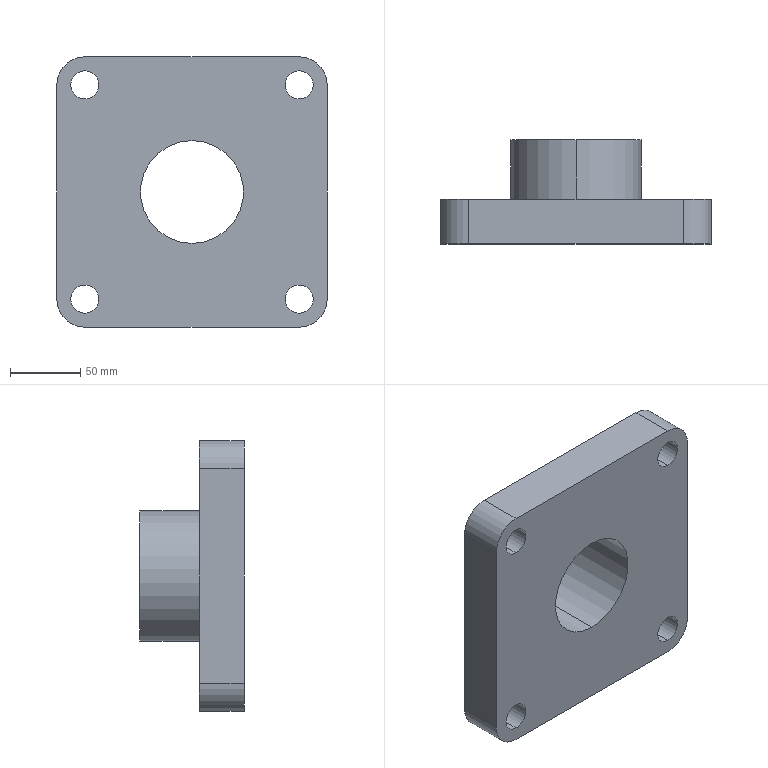Part | SolidWorks | features BaseBody 1 | 1 solid | 23 faces | box 193 x 74.6 x 193 mm | volume 1117041 mm3 | cylinder 16 | plane 7 | commonest cylinder face diameters 20 x8 40 x4 73.374 x2 93.374 x2
STEP:
#1=CARTESIAN_POINT('',(0.,74.6,-36.687));
#2=VERTEX_POINT('',#1);
#3=CARTESIAN_POINT('',(0.,74.6,36.687));
#4=VERTEX_POINT('',#3);
#5=CARTESIAN_POINT('',(0.,74.6,0.));
#6=DIRECTION('',(0.,1.,0.));
#7=DIRECTION('',(0.,0.,1.));
#8=AXIS2_PLACEMENT_3D('',#5,#6,#7);
#9=CIRCLE('',#8,36.687);
#10=EDGE_CURVE('',#2,#4,#9,.T.);
#11=ORIENTED_EDGE('',*,*,#10,.T.);
#12=CARTESIAN_POINT('',(0.,0.,36.687));
#13=VERTEX_POINT('',#12);
#14=CARTESIAN_POINT('',(0.,74.6,36.687));
#15=DIRECTION('',(0.,-1.,0.));
#16=VECTOR('',#15,1000.);
#17=LINE('',#14,#16);
#18=EDGE_CURVE('',#4,#13,#17,.T.);
#19=ORIENTED_EDGE('',*,*,#18,.T.);
#20=CARTESIAN_POINT('',(0.,0.,-36.687));
#21=VERTEX_POINT('',#20);
#22=CARTESIAN_POINT('',(0.,0.,0.));
#23=DIRECTION('',(0.,1.,0.));
#24=DIRECTION('',(0.,0.,1.));
#25=AXIS2_PLACEMENT_3D('',#22,#23,#24);
#26=CIRCLE('',#25,36.687);
#27=EDGE_CURVE('',#21,#13,#26,.T.);
#28=ORIENTED_EDGE('',*,*,#27,.F.);
#29=CARTESIAN_POINT('',(0.,74.6,-36.687));
#30=DIRECTION('',(0.,-1.,0.));
#31=VECTOR('',#30,1000.);
#32=LINE('',#29,#31);
#33=EDGE_CURVE('',#2,#21,#32,.T.);
#34=ORIENTED_EDGE('',*,*,#33,.F.);
#35=EDGE_LOOP('',(#11,#19,#28,#34));
#36=FACE_OUTER_BOUND('',#35,.T.);
#37=CARTESIAN_POINT('',(0.,74.6,0.));
#38=DIRECTION('',(0.,-1.,0.));
#39=DIRECTION('',(0.,0.,-1.));
#40=AXIS2_PLACEMENT_3D('',#37,#38,#39);
#41=CYLINDRICAL_SURFACE('',#40,36.687);
#42=ADVANCED_FACE('',(#36),#41,.F.);
#43=CARTESIAN_POINT('',(0.,74.6,46.687));
#44=VERTEX_POINT('',#43);
#45=CARTESIAN_POINT('',(0.,74.6,-46.687));
#46=VERTEX_POINT('',#45);
#47=CARTESIAN_POINT('',(0.,74.6,0.));
#48=DIRECTION('',(0.,1.,0.));
#49=DIRECTION('',(0.,0.,1.));
#50=AXIS2_PLACEMENT_3D('',#47,#48,#49);
#51=CIRCLE('',#50,46.687);
#52=EDGE_CURVE('',#44,#46,#51,.T.);
#53=ORIENTED_EDGE('',*,*,#52,.F.);
#54=CARTESIAN_POINT('',(0.,32.,46.687));
#55=VERTEX_POINT('',#54);
#56=CARTESIAN_POINT('',(0.,74.6,46.687));
#57=DIRECTION('',(0.,-1.,0.));
#58=VECTOR('',#57,1000.);
#59=LINE('',#56,#58);
#60=EDGE_CURVE('',#44,#55,#59,.T.);
#61=ORIENTED_EDGE('',*,*,#60,.T.);
#62=CARTESIAN_POINT('',(0.,32.,-46.687));
#63=VERTEX_POINT('',#62);
#64=CARTESIAN_POINT('',(0.,32.,0.));
#65=DIRECTION('',(0.,-1.,0.));
#66=DIRECTION('',(0.,0.,1.));
#67=AXIS2_PLACEMENT_3D('',#64,#65,#66);
#68=CIRCLE('',#67,46.687);
#69=EDGE_CURVE('',#63,#55,#68,.T.);
#70=ORIENTED_EDGE('',*,*,#69,.F.);
#71=CARTESIAN_POINT('',(0.,74.6,-46.687));
#72=DIRECTION('',(0.,-1.,0.));
#73=VECTOR('',#72,1000.);
#74=LINE('',#71,#73);
#75=EDGE_CURVE('',#46,#63,#74,.T.);
#76=ORIENTED_EDGE('',*,*,#75,.F.);
#77=EDGE_LOOP('',(#53,#61,#70,#76));
#78=FACE_OUTER_BOUND('',#77,.T.);
#79=CARTESIAN_POINT('',(0.,74.6,0.));
#80=DIRECTION('',(0.,-1.,0.));
#81=DIRECTION('',(0.,0.,-1.));
#82=AXIS2_PLACEMENT_3D('',#79,#80,#81);
#83=CYLINDRICAL_SURFACE('',#82,46.687);
#84=ADVANCED_FACE('',(#78),#83,.T.);
#85=CARTESIAN_POINT('',(76.5,32.,66.5));
#86=VERTEX_POINT('',#85);
#87=CARTESIAN_POINT('',(76.5,32.,86.5));
#88=VERTEX_POINT('',#87);
#89=CARTESIAN_POINT('',(76.5,32.,76.5));
#90=DIRECTION('',(0.,1.,0.));
#91=DIRECTION('',(0.,0.,1.));
#92=AXIS2_PLACEMENT_3D('',#89,#90,#91);
#93=CIRCLE('',#92,10.);
#94=EDGE_CURVE('',#86,#88,#93,.T.);
#95=ORIENTED_EDGE('',*,*,#94,.T.);
#96=CARTESIAN_POINT('',(76.5,0.,86.5));
#97=VERTEX_POINT('',#96);
#98=CARTESIAN_POINT('',(76.5,32.,86.5));
#99=DIRECTION('',(0.,-1.,0.));
#100=VECTOR('',#99,1000.);
#101=LINE('',#98,#100);
#102=EDGE_CURVE('',#88,#97,#101,.T.);
#103=ORIENTED_EDGE('',*,*,#102,.T.);
#104=CARTESIAN_POINT('',(76.5,0.,66.5));
#105=VERTEX_POINT('',#104);
#106=CARTESIAN_POINT('',(76.5,0.,76.5));
#107=DIRECTION('',(0.,1.,0.));
#108=DIRECTION('',(0.,0.,1.));
#109=AXIS2_PLACEMENT_3D('',#106,#107,#108);
#110=CIRCLE('',#109,10.);
#111=EDGE_CURVE('',#105,#97,#110,.T.);
#112=ORIENTED_EDGE('',*,*,#111,.F.);
#113=CARTESIAN_POINT('',(76.5,32.,66.5));
#114=DIRECTION('',(0.,-1.,0.));
#115=VECTOR('',#114,1000.);
#116=LINE('',#113,#115);
#117=EDGE_CURVE('',#86,#105,#116,.T.);
#118=ORIENTED_EDGE('',*,*,#117,.F.);
#119=EDGE_LOOP('',(#95,#103,#112,#118));
#120=FACE_OUTER_BOUND('',#119,.T.);
#121=CARTESIAN_POINT('',(76.5,32.,76.5));
#122=DIRECTION('',(0.,-1.,0.));
#123=DIRECTION('',(0.,0.,-1.));
#124=AXIS2_PLACEMENT_3D('',#121,#122,#123);
#125=CYLINDRICAL_SURFACE('',#124,10.);
#126=ADVANCED_FACE('',(#120),#125,.F.);
#127=CARTESIAN_POINT('',(76.5,32.,-86.5));
#128=VERTEX_POINT('',#127);
#129=CARTESIAN_POINT('',(76.5,32.,-66.5));
#130=VERTEX_POINT('',#129);
#131=CARTESIAN_POINT('',(76.5,32.,-76.5));
#132=DIRECTION('',(0.,1.,0.));
#133=DIRECTION('',(0.,0.,1.));
#134=AXIS2_PLACEMENT_3D('',#131,#132,#133);
#135=CIRCLE('',#134,10.);
#136=EDGE_CURVE('',#128,#130,#135,.T.);
#137=ORIENTED_EDGE('',*,*,#136,.T.);
#138=CARTESIAN_POINT('',(76.5,0.,-66.5));
#139=VERTEX_POINT('',#138);
#140=CARTESIAN_POINT('',(76.5,32.,-66.5));
#141=DIRECTION('',(0.,-1.,0.));
#142=VECTOR('',#141,1000.);
#143=LINE('',#140,#142);
#144=EDGE_CURVE('',#130,#139,#143,.T.);
#145=ORIENTED_EDGE('',*,*,#144,.T.);
#146=CARTESIAN_POINT('',(76.5,0.,-86.5));
#147=VERTEX_POINT('',#146);
#148=CARTESIAN_POINT('',(76.5,0.,-76.5));
#149=DIRECTION('',(0.,1.,0.));
#150=DIRECTION('',(0.,0.,1.));
#151=AXIS2_PLACEMENT_3D('',#148,#149,#150);
#152=CIRCLE('',#151,10.);
#153=EDGE_CURVE('',#147,#139,#152,.T.);
#154=ORIENTED_EDGE('',*,*,#153,.F.);
#155=CARTESIAN_POINT('',(76.5,32.,-86.5));
#156=DIRECTION('',(0.,-1.,0.));
#157=VECTOR('',#156,1000.);
#158=LINE('',#155,#157);
#159=EDGE_CURVE('',#128,#147,#158,.T.);
#160=ORIENTED_EDGE('',*,*,#159,.F.);
#161=EDGE_LOOP('',(#137,#145,#154,#160));
#162=FACE_OUTER_BOUND('',#161,.T.);
#163=CARTESIAN_POINT('',(76.5,32.,-76.5));
#164=DIRECTION('',(0.,-1.,0.));
#165=DIRECTION('',(0.,0.,-1.));
#166=AXIS2_PLACEMENT_3D('',#163,#164,#165);
#167=CYLINDRICAL_SURFACE('',#166,10.);
#168=ADVANCED_FACE('',(#162),#167,.F.);
#169=CARTESIAN_POINT('',(-76.5,32.,66.5));
#170=VERTEX_POINT('',#169);
#171=CARTESIAN_POINT('',(-76.5,32.,86.5));
#172=VERTEX_POINT('',#171);
#173=CARTESIAN_POINT('',(-76.5,32.,76.5));
#174=DIRECTION('',(0.,1.,0.));
#175=DIRECTION('',(0.,0.,1.));
#176=AXIS2_PLACEMENT_3D('',#173,#174,#175);
#177=CIRCLE('',#176,10.);
#178=EDGE_CURVE('',#170,#172,#177,.T.);
#179=ORIENTED_EDGE('',*,*,#178,.T.);
#180=CARTESIAN_POINT('',(-76.5,0.,86.5));
#181=VERTEX_POINT('',#180);
#182=CARTESIAN_POINT('',(-76.5,32.,86.5));
#183=DIRECTION('',(0.,-1.,0.));
#184=VECTOR('',#183,1000.);
#185=LINE('',#182,#184);
#186=EDGE_CURVE('',#172,#181,#185,.T.);
#187=ORIENTED_EDGE('',*,*,#186,.T.);
#188=CARTESIAN_POINT('',(-76.5,0.,66.5));
#189=VERTEX_POINT('',#188);
#190=CARTESIAN_POINT('',(-76.5,0.,76.5));
#191=DIRECTION('',(0.,1.,0.));
#192=DIRECTION('',(0.,0.,1.));
#193=AXIS2_PLACEMENT_3D('',#190,#191,#192);
#194=CIRCLE('',#193,10.);
#195=EDGE_CURVE('',#189,#181,#194,.T.);
#196=ORIENTED_EDGE('',*,*,#195,.F.);
#197=CARTESIAN_POINT('',(-76.5,32.,66.5));
#198=DIRECTION('',(0.,-1.,0.));
#199=VECTOR('',#198,1000.);
#200=LINE('',#197,#199);
#201=EDGE_CURVE('',#170,#189,#200,.T.);
#202=ORIENTED_EDGE('',*,*,#201,.F.);
#203=EDGE_LOOP('',(#179,#187,#196,#202));
#204=FACE_OUTER_BOUND('',#203,.T.);
#205=CARTESIAN_POINT('',(-76.5,32.,76.5));
#206=DIRECTION('',(0.,-1.,0.));
#207=DIRECTION('',(0.,0.,-1.));
#208=AXIS2_PLACEMENT_3D('',#205,#206,#207);
#209=CYLINDRICAL_SURFACE('',#208,10.);
#210=ADVANCED_FACE('',(#204),#209,.F.);
#211=CARTESIAN_POINT('',(-76.5,32.,-86.5));
#212=VERTEX_POINT('',#211);
#213=CARTESIAN_POINT('',(-76.5,32.,-66.5));
#214=VERTEX_POINT('',#213);
#215=CARTESIAN_POINT('',(-76.5,32.,-76.5));
#216=DIRECTION('',(0.,1.,0.));
#217=DIRECTION('',(0.,0.,1.));
#218=AXIS2_PLACEMENT_3D('',#215,#216,#217);
#219=CIRCLE('',#218,10.);
#220=EDGE_CURVE('',#212,#214,#219,.T.);
#221=ORIENTED_EDGE('',*,*,#220,.T.);
#222=CARTESIAN_POINT('',(-76.5,0.,-66.5));
#223=VERTEX_POINT('',#222);
#224=CARTESIAN_POINT('',(-76.5,32.,-66.5));
#225=DIRECTION('',(0.,-1.,0.));
#226=VECTOR('',#225,1000.);
#227=LINE('',#224,#226);
#228=EDGE_CURVE('',#214,#223,#227,.T.);
#229=ORIENTED_EDGE('',*,*,#228,.T.);
#230=CARTESIAN_POINT('',(-76.5,0.,-86.5));
#231=VERTEX_POINT('',#230);
#232=CARTESIAN_POINT('',(-76.5,0.,-76.5));
#233=DIRECTION('',(0.,1.,0.));
#234=DIRECTION('',(0.,0.,1.));
#235=AXIS2_PLACEMENT_3D('',#232,#233,#234);
#236=CIRCLE('',#235,10.);
#237=EDGE_CURVE('',#231,#223,#236,.T.);
#238=ORIENTED_EDGE('',*,*,#237,.F.);
#239=CARTESIAN_POINT('',(-76.5,32.,-86.5));
#240=DIRECTION('',(0.,-1.,0.));
#241=VECTOR('',#240,1000.);
#242=LINE('',#239,#241);
#243=EDGE_CURVE('',#212,#231,#242,.T.);
#244=ORIENTED_EDGE('',*,*,#243,.F.);
#245=EDGE_LOOP('',(#221,#229,#238,#244));
#246=FACE_OUTER_BOUND('',#245,.T.);
#247=CARTESIAN_POINT('',(-76.5,32.,-76.5));
#248=DIRECTION('',(0.,-1.,0.));
#249=DIRECTION('',(0.,0.,-1.));
#250=AXIS2_PLACEMENT_3D('',#247,#248,#249);
#251=CYLINDRICAL_SURFACE('',#250,10.);
#252=ADVANCED_FACE('',(#246),#251,.F.);
#253=ORIENTED_EDGE('',*,*,#69,.T.);
#254=CARTESIAN_POINT('',(0.,32.,0.));
#255=DIRECTION('',(0.,-1.,0.));
#256=DIRECTION('',(0.,0.,1.));
#257=AXIS2_PLACEMENT_3D('',#254,#255,#256);
#258=CIRCLE('',#257,46.687);
#259=EDGE_CURVE('',#55,#63,#258,.T.);
#260=ORIENTED_EDGE('',*,*,#259,.T.);
#261=EDGE_LOOP('',(#253,#260));
#262=FACE_BOUND('',#261,.T.);
#263=ORIENTED_EDGE('',*,*,#136,.F.);
#264=CARTESIAN_POINT('',(76.5,32.,-76.5));
#265=DIRECTION('',(0.,1.,0.));
#266=DIRECTION('',(0.,0.,1.));
#267=AXIS2_PLACEMENT_3D('',#264,#265,#266);
#268=CIRCLE('',#267,10.);
#269=EDGE_CURVE('',#130,#128,#268,.T.);
#270=ORIENTED_EDGE('',*,*,#269,.F.);
#271=EDGE_LOOP('',(#263,#270));
#272=FACE_BOUND('',#271,.T.);
#273=ORIENTED_EDGE('',*,*,#220,.F.);
#274=CARTESIAN_POINT('',(-76.5,32.,-76.5));
#275=DIRECTION('',(0.,1.,0.));
#276=DIRECTION('',(0.,0.,1.));
#277=AXIS2_PLACEMENT_3D('',#274,#275,#276);
#278=CIRCLE('',#277,10.);
#279=EDGE_CURVE('',#214,#212,#278,.T.);
#280=ORIENTED_EDGE('',*,*,#279,.F.);
#281=EDGE_LOOP('',(#273,#280));
#282=FACE_BOUND('',#281,.T.);
#283=CARTESIAN_POINT('',(-76.5,32.,-96.5));
#284=VERTEX_POINT('',#283);
#285=CARTESIAN_POINT('',(-96.5,32.,-76.5));
#286=VERTEX_POINT('',#285);
#287=CARTESIAN_POINT('',(-76.5,32.,-76.5));
#288=DIRECTION('',(0.,1.,0.));
#289=DIRECTION('',(0.,0.,1.));
#290=AXIS2_PLACEMENT_3D('',#287,#288,#289);
#291=CIRCLE('',#290,20.);
#292=EDGE_CURVE('',#284,#286,#291,.T.);
#293=ORIENTED_EDGE('',*,*,#292,.T.);
#294=CARTESIAN_POINT('',(-96.5,32.,76.5));
#295=VERTEX_POINT('',#294);
#296=CARTESIAN_POINT('',(-96.5,32.,-76.5));
#297=DIRECTION('',(0.,0.,1.));
#298=VECTOR('',#297,1000.);
#299=LINE('',#296,#298);
#300=EDGE_CURVE('',#286,#295,#299,.T.);
#301=ORIENTED_EDGE('',*,*,#300,.T.);
#302=CARTESIAN_POINT('',(-76.5,32.,96.5));
#303=VERTEX_POINT('',#302);
#304=CARTESIAN_POINT('',(-76.5,32.,76.5));
#305=DIRECTION('',(0.,1.,0.));
#306=DIRECTION('',(0.,0.,-1.));
#307=AXIS2_PLACEMENT_3D('',#304,#305,#306);
#308=CIRCLE('',#307,20.);
#309=EDGE_CURVE('',#295,#303,#308,.T.);
#310=ORIENTED_EDGE('',*,*,#309,.T.);
#311=CARTESIAN_POINT('',(76.5,32.,96.5));
#312=VERTEX_POINT('',#311);
#313=CARTESIAN_POINT('',(-76.5,32.,96.5));
#314=DIRECTION('',(1.,0.,0.));
#315=VECTOR('',#314,1000.);
#316=LINE('',#313,#315);
#317=EDGE_CURVE('',#303,#312,#316,.T.);
#318=ORIENTED_EDGE('',*,*,#317,.T.);
#319=CARTESIAN_POINT('',(96.5,32.,76.5));
#320=VERTEX_POINT('',#319);
#321=CARTESIAN_POINT('',(76.5,32.,76.5));
#322=DIRECTION('',(0.,1.,0.));
#323=DIRECTION('',(0.,0.,1.));
#324=AXIS2_PLACEMENT_3D('',#321,#322,#323);
#325=CIRCLE('',#324,20.);
#326=EDGE_CURVE('',#312,#320,#325,.T.);
#327=ORIENTED_EDGE('',*,*,#326,.T.);
#328=CARTESIAN_POINT('',(96.5,32.,-76.5));
#329=VERTEX_POINT('',#328);
#330=CARTESIAN_POINT('',(96.5,32.,-76.5));
#331=DIRECTION('',(0.,0.,-1.));
#332=VECTOR('',#331,1000.);
#333=LINE('',#330,#332);
#334=EDGE_CURVE('',#320,#329,#333,.T.);
#335=ORIENTED_EDGE('',*,*,#334,.T.);
#336=CARTESIAN_POINT('',(76.5,32.,-96.5));
#337=VERTEX_POINT('',#336);
#338=CARTESIAN_POINT('',(76.5,32.,-76.5));
#339=DIRECTION('',(0.,1.,0.));
#340=DIRECTION('',(0.,0.,1.));
#341=AXIS2_PLACEMENT_3D('',#338,#339,#340);
#342=CIRCLE('',#341,20.);
#343=EDGE_CURVE('',#329,#337,#342,.T.);
#344=ORIENTED_EDGE('',*,*,#343,.T.);
#345=CARTESIAN_POINT('',(-76.5,32.,-96.5));
#346=DIRECTION('',(-1.,0.,0.));
#347=VECTOR('',#346,1000.);
#348=LINE('',#345,#347);
#349=EDGE_CURVE('',#337,#284,#348,.T.);
#350=ORIENTED_EDGE('',*,*,#349,.T.);
#351=EDGE_LOOP('',(#293,#301,#310,#318,#327,#335,#344,#350));
#352=FACE_OUTER_BOUND('',#351,.T.);
#353=ORIENTED_EDGE('',*,*,#178,.F.);
#354=CARTESIAN_POINT('',(-76.5,32.,76.5));
#355=DIRECTION('',(0.,1.,0.));
#356=DIRECTION('',(0.,0.,1.));
#357=AXIS2_PLACEMENT_3D('',#354,#355,#356);
#358=CIRCLE('',#357,10.);
#359=EDGE_CURVE('',#172,#170,#358,.T.);
#360=ORIENTED_EDGE('',*,*,#359,.F.);
#361=EDGE_LOOP('',(#353,#360));
#362=FACE_BOUND('',#361,.T.);
#363=ORIENTED_EDGE('',*,*,#94,.F.);
#364=CARTESIAN_POINT('',(76.5,32.,76.5));
#365=DIRECTION('',(0.,1.,0.));
#366=DIRECTION('',(0.,0.,1.));
#367=AXIS2_PLACEMENT_3D('',#364,#365,#366);
#368=CIRCLE('',#367,10.);
#369=EDGE_CURVE('',#88,#86,#368,.T.);
#370=ORIENTED_EDGE('',*,*,#369,.F.);
#371=EDGE_LOOP('',(#363,#370));
#372=FACE_BOUND('',#371,.T.);
#373=CARTESIAN_POINT('',(-76.5,32.,-76.5));
#374=DIRECTION('',(0.,1.,0.));
#375=DIRECTION('',(0.,0.,1.));
#376=AXIS2_PLACEMENT_3D('',#373,#374,#375);
#377=PLANE('',#376);
#378=ADVANCED_FACE('',(#262,#272,#282,#352,#362,#372),#377,.T.);
#379=ORIENTED_EDGE('',*,*,#27,.T.);
#380=CARTESIAN_POINT('',(0.,0.,0.));
#381=DIRECTION('',(0.,1.,0.));
#382=DIRECTION('',(0.,0.,1.));
#383=AXIS2_PLACEMENT_3D('',#380,#381,#382);
#384=CIRCLE('',#383,36.687);
#385=EDGE_CURVE('',#13,#21,#384,.T.);
#386=ORIENTED_EDGE('',*,*,#385,.T.);
#387=EDGE_LOOP('',(#379,#386));
#388=FACE_BOUND('',#387,.T.);
#389=CARTESIAN_POINT('',(-76.5,0.,-96.5));
#390=VERTEX_POINT('',#389);
#391=CARTESIAN_POINT('',(-96.5,0.,-76.5));
#392=VERTEX_POINT('',#391);
#393=CARTESIAN_POINT('',(-76.5,0.,-76.5));
#394=DIRECTION('',(0.,1.,0.));
#395=DIRECTION('',(0.,0.,1.));
#396=AXIS2_PLACEMENT_3D('',#393,#394,#395);
#397=CIRCLE('',#396,20.);
#398=EDGE_CURVE('',#390,#392,#397,.T.);
#399=ORIENTED_EDGE('',*,*,#398,.F.);
#400=CARTESIAN_POINT('',(76.5,0.,-96.5));
#401=VERTEX_POINT('',#400);
#402=CARTESIAN_POINT('',(-76.5,0.,-96.5));
#403=DIRECTION('',(-1.,0.,0.));
#404=VECTOR('',#403,1000.);
#405=LINE('',#402,#404);
#406=EDGE_CURVE('',#401,#390,#405,.T.);
#407=ORIENTED_EDGE('',*,*,#406,.F.);
#408=CARTESIAN_POINT('',(96.5,0.,-76.5));
#409=VERTEX_POINT('',#408);
#410=CARTESIAN_POINT('',(76.5,0.,-76.5));
#411=DIRECTION('',(0.,1.,0.));
#412=DIRECTION('',(0.,0.,1.));
#413=AXIS2_PLACEMENT_3D('',#410,#411,#412);
#414=CIRCLE('',#413,20.);
#415=EDGE_CURVE('',#409,#401,#414,.T.);
#416=ORIENTED_EDGE('',*,*,#415,.F.);
#417=CARTESIAN_POINT('',(96.5,0.,76.5));
#418=VERTEX_POINT('',#417);
#419=CARTESIAN_POINT('',(96.5,0.,-76.5));
#420=DIRECTION('',(0.,0.,-1.));
#421=VECTOR('',#420,1000.);
#422=LINE('',#419,#421);
#423=EDGE_CURVE('',#418,#409,#422,.T.);
#424=ORIENTED_EDGE('',*,*,#423,.F.);
#425=CARTESIAN_POINT('',(76.5,0.,96.5));
#426=VERTEX_POINT('',#425);
#427=CARTESIAN_POINT('',(76.5,0.,76.5));
#428=DIRECTION('',(0.,1.,0.));
#429=DIRECTION('',(0.,0.,1.));
#430=AXIS2_PLACEMENT_3D('',#427,#428,#429);
#431=CIRCLE('',#430,20.);
#432=EDGE_CURVE('',#426,#418,#431,.T.);
#433=ORIENTED_EDGE('',*,*,#432,.F.);
#434=CARTESIAN_POINT('',(-76.5,0.,96.5));
#435=VERTEX_POINT('',#434);
#436=CARTESIAN_POINT('',(-76.5,0.,96.5));
#437=DIRECTION('',(1.,0.,0.));
#438=VECTOR('',#437,1000.);
#439=LINE('',#436,#438);
#440=EDGE_CURVE('',#435,#426,#439,.T.);
#441=ORIENTED_EDGE('',*,*,#440,.F.);
#442=CARTESIAN_POINT('',(-96.5,0.,76.5));
#443=VERTEX_POINT('',#442);
#444=CARTESIAN_POINT('',(-76.5,0.,76.5));
#445=DIRECTION('',(0.,1.,0.));
#446=DIRECTION('',(0.,0.,-1.));
#447=AXIS2_PLACEMENT_3D('',#444,#445,#446);
#448=CIRCLE('',#447,20.);
#449=EDGE_CURVE('',#443,#435,#448,.T.);
#450=ORIENTED_EDGE('',*,*,#449,.F.);
#451=CARTESIAN_POINT('',(-96.5,0.,-76.5));
#452=DIRECTION('',(0.,0.,1.));
#453=VECTOR('',#452,1000.);
#454=LINE('',#451,#453);
#455=EDGE_CURVE('',#392,#443,#454,.T.);
#456=ORIENTED_EDGE('',*,*,#455,.F.);
#457=EDGE_LOOP('',(#399,#407,#416,#424,#433,#441,#450,#456));
#458=FACE_OUTER_BOUND('',#457,.T.);
#459=ORIENTED_EDGE('',*,*,#237,.T.);
#460=CARTESIAN_POINT('',(-76.5,0.,-76.5));
#461=DIRECTION('',(0.,1.,0.));
#462=DIRECTION('',(0.,0.,1.));
#463=AXIS2_PLACEMENT_3D('',#460,#461,#462);
#464=CIRCLE('',#463,10.);
#465=EDGE_CURVE('',#223,#231,#464,.T.);
#466=ORIENTED_EDGE('',*,*,#465,.T.);
#467=EDGE_LOOP('',(#459,#466));
#468=FACE_BOUND('',#467,.T.);
#469=ORIENTED_EDGE('',*,*,#195,.T.);
#470=CARTESIAN_POINT('',(-76.5,0.,76.5));
#471=DIRECTION('',(0.,1.,0.));
#472=DIRECTION('',(0.,0.,1.));
#473=AXIS2_PLACEMENT_3D('',#470,#471,#472);
#474=CIRCLE('',#473,10.);
#475=EDGE_CURVE('',#181,#189,#474,.T.);
#476=ORIENTED_EDGE('',*,*,#475,.T.);
#477=EDGE_LOOP('',(#469,#476));
#478=FACE_BOUND('',#477,.T.);
#479=ORIENTED_EDGE('',*,*,#153,.T.);
#480=CARTESIAN_POINT('',(76.5,0.,-76.5));
#481=DIRECTION('',(0.,1.,0.));
#482=DIRECTION('',(0.,0.,1.));
#483=AXIS2_PLACEMENT_3D('',#480,#481,#482);
#484=CIRCLE('',#483,10.);
#485=EDGE_CURVE('',#139,#147,#484,.T.);
#486=ORIENTED_EDGE('',*,*,#485,.T.);
#487=EDGE_LOOP('',(#479,#486));
#488=FACE_BOUND('',#487,.T.);
#489=ORIENTED_EDGE('',*,*,#111,.T.);
#490=CARTESIAN_POINT('',(76.5,0.,76.5));
#491=DIRECTION('',(0.,1.,0.));
#492=DIRECTION('',(0.,0.,1.));
#493=AXIS2_PLACEMENT_3D('',#490,#491,#492);
#494=CIRCLE('',#493,10.);
#495=EDGE_CURVE('',#97,#105,#494,.T.);
#496=ORIENTED_EDGE('',*,*,#495,.T.);
#497=EDGE_LOOP('',(#489,#496));
#498=FACE_BOUND('',#497,.T.);
#499=CARTESIAN_POINT('',(-76.5,0.,-76.5));
#500=DIRECTION('',(0.,1.,0.));
#501=DIRECTION('',(0.,0.,1.));
#502=AXIS2_PLACEMENT_3D('',#499,#500,#501);
#503=PLANE('',#502);
#504=ADVANCED_FACE('',(#388,#458,#468,#478,#488,#498),#503,.F.);
#505=ORIENTED_EDGE('',*,*,#398,.T.);
#506=CARTESIAN_POINT('',(-96.5,32.,-76.5));
#507=DIRECTION('',(0.,-1.,0.));
#508=VECTOR('',#507,1000.);
#509=LINE('',#506,#508);
#510=EDGE_CURVE('',#286,#392,#509,.T.);
#511=ORIENTED_EDGE('',*,*,#510,.F.);
#512=ORIENTED_EDGE('',*,*,#292,.F.);
#513=CARTESIAN_POINT('',(-76.5,32.,-96.5));
#514=DIRECTION('',(0.,-1.,0.));
#515=VECTOR('',#514,1000.);
#516=LINE('',#513,#515);
#517=EDGE_CURVE('',#284,#390,#516,.T.);
#518=ORIENTED_EDGE('',*,*,#517,.T.);
#519=EDGE_LOOP('',(#505,#511,#512,#518));
#520=FACE_OUTER_BOUND('',#519,.T.);
#521=CARTESIAN_POINT('',(-76.5,32.,-76.5));
#522=DIRECTION('',(0.,-1.,0.));
#523=DIRECTION('',(0.,0.,-1.));
#524=AXIS2_PLACEMENT_3D('',#521,#522,#523);
#525=CYLINDRICAL_SURFACE('',#524,20.);
#526=ADVANCED_FACE('',(#520),#525,.T.);
#527=ORIENTED_EDGE('',*,*,#455,.T.);
#528=CARTESIAN_POINT('',(-96.5,32.,76.5));
#529=DIRECTION('',(0.,-1.,0.));
#530=VECTOR('',#529,1000.);
#531=LINE('',#528,#530);
#532=EDGE_CURVE('',#295,#443,#531,.T.);
#533=ORIENTED_EDGE('',*,*,#532,.F.);
#534=ORIENTED_EDGE('',*,*,#300,.F.);
#535=ORIENTED_EDGE('',*,*,#510,.T.);
#536=EDGE_LOOP('',(#527,#533,#534,#535));
#537=FACE_OUTER_BOUND('',#536,.T.);
#538=CARTESIAN_POINT('',(-96.5,32.,-76.5));
#539=DIRECTION('',(1.,0.,0.));
#540=DIRECTION('',(0.,0.,-1.));
#541=AXIS2_PLACEMENT_3D('',#538,#539,#540);
#542=PLANE('',#541);
#543=ADVANCED_FACE('',(#537),#542,.F.);
#544=ORIENTED_EDGE('',*,*,#449,.T.);
#545=CARTESIAN_POINT('',(-76.5,32.,96.5));
#546=DIRECTION('',(0.,-1.,0.));
#547=VECTOR('',#546,1000.);
#548=LINE('',#545,#547);
#549=EDGE_CURVE('',#303,#435,#548,.T.);
#550=ORIENTED_EDGE('',*,*,#549,.F.);
#551=ORIENTED_EDGE('',*,*,#309,.F.);
#552=ORIENTED_EDGE('',*,*,#532,.T.);
#553=EDGE_LOOP('',(#544,#550,#551,#552));
#554=FACE_OUTER_BOUND('',#553,.T.);
#555=CARTESIAN_POINT('',(-76.5,32.,76.5));
#556=DIRECTION('',(0.,-1.,0.));
#557=DIRECTION('',(0.,0.,-1.));
#558=AXIS2_PLACEMENT_3D('',#555,#556,#557);
#559=CYLINDRICAL_SURFACE('',#558,20.);
#560=ADVANCED_FACE('',(#554),#559,.T.);
#561=ORIENTED_EDGE('',*,*,#440,.T.);
#562=CARTESIAN_POINT('',(76.5,32.,96.5));
#563=DIRECTION('',(0.,-1.,0.));
#564=VECTOR('',#563,1000.);
#565=LINE('',#562,#564);
#566=EDGE_CURVE('',#312,#426,#565,.T.);
#567=ORIENTED_EDGE('',*,*,#566,.F.);
#568=ORIENTED_EDGE('',*,*,#317,.F.);
#569=ORIENTED_EDGE('',*,*,#549,.T.);
#570=EDGE_LOOP('',(#561,#567,#568,#569));
#571=FACE_OUTER_BOUND('',#570,.T.);
#572=CARTESIAN_POINT('',(-76.5,32.,96.5));
#573=DIRECTION('',(0.,0.,-1.));
#574=DIRECTION('',(-1.,0.,0.));
#575=AXIS2_PLACEMENT_3D('',#572,#573,#574);
#576=PLANE('',#575);
#577=ADVANCED_FACE('',(#571),#576,.F.);
#578=ORIENTED_EDGE('',*,*,#432,.T.);
#579=CARTESIAN_POINT('',(96.5,32.,76.5));
#580=DIRECTION('',(0.,-1.,0.));
#581=VECTOR('',#580,1000.);
#582=LINE('',#579,#581);
#583=EDGE_CURVE('',#320,#418,#582,.T.);
#584=ORIENTED_EDGE('',*,*,#583,.F.);
#585=ORIENTED_EDGE('',*,*,#326,.F.);
#586=ORIENTED_EDGE('',*,*,#566,.T.);
#587=EDGE_LOOP('',(#578,#584,#585,#586));
#588=FACE_OUTER_BOUND('',#587,.T.);
#589=CARTESIAN_POINT('',(76.5,32.,76.5));
#590=DIRECTION('',(0.,-1.,0.));
#591=DIRECTION('',(0.,0.,-1.));
#592=AXIS2_PLACEMENT_3D('',#589,#590,#591);
#593=CYLINDRICAL_SURFACE('',#592,20.);
#594=ADVANCED_FACE('',(#588),#593,.T.);
#595=ORIENTED_EDGE('',*,*,#423,.T.);
#596=CARTESIAN_POINT('',(96.5,32.,-76.5));
#597=DIRECTION('',(0.,-1.,0.));
#598=VECTOR('',#597,1000.);
#599=LINE('',#596,#598);
#600=EDGE_CURVE('',#329,#409,#599,.T.);
#601=ORIENTED_EDGE('',*,*,#600,.F.);
#602=ORIENTED_EDGE('',*,*,#334,.F.);
#603=ORIENTED_EDGE('',*,*,#583,.T.);
#604=EDGE_LOOP('',(#595,#601,#602,#603));
#605=FACE_OUTER_BOUND('',#604,.T.);
#606=CARTESIAN_POINT('',(96.5,32.,-76.5));
#607=DIRECTION('',(-1.,0.,0.));
#608=DIRECTION('',(0.,0.,1.));
#609=AXIS2_PLACEMENT_3D('',#606,#607,#608);
#610=PLANE('',#609);
#611=ADVANCED_FACE('',(#605),#610,.F.);
#612=ORIENTED_EDGE('',*,*,#415,.T.);
#613=CARTESIAN_POINT('',(76.5,32.,-96.5));
#614=DIRECTION('',(0.,-1.,0.));
#615=VECTOR('',#614,1000.);
#616=LINE('',#613,#615);
#617=EDGE_CURVE('',#337,#401,#616,.T.);
#618=ORIENTED_EDGE('',*,*,#617,.F.);
#619=ORIENTED_EDGE('',*,*,#343,.F.);
#620=ORIENTED_EDGE('',*,*,#600,.T.);
#621=EDGE_LOOP('',(#612,#618,#619,#620));
#622=FACE_OUTER_BOUND('',#621,.T.);
#623=CARTESIAN_POINT('',(76.5,32.,-76.5));
#624=DIRECTION('',(0.,-1.,0.));
#625=DIRECTION('',(0.,0.,-1.));
#626=AXIS2_PLACEMENT_3D('',#623,#624,#625);
#627=CYLINDRICAL_SURFACE('',#626,20.);
#628=ADVANCED_FACE('',(#622),#627,.T.);
#629=ORIENTED_EDGE('',*,*,#406,.T.);
#630=ORIENTED_EDGE('',*,*,#517,.F.);
#631=ORIENTED_EDGE('',*,*,#349,.F.);
#632=ORIENTED_EDGE('',*,*,#617,.T.);
#633=EDGE_LOOP('',(#629,#630,#631,#632));
#634=FACE_OUTER_BOUND('',#633,.T.);
#635=CARTESIAN_POINT('',(-76.5,32.,-96.5));
#636=DIRECTION('',(0.,0.,1.));
#637=DIRECTION('',(1.,0.,0.));
#638=AXIS2_PLACEMENT_3D('',#635,#636,#637);
#639=PLANE('',#638);
#640=ADVANCED_FACE('',(#634),#639,.F.);
#641=ORIENTED_EDGE('',*,*,#228,.F.);
#642=ORIENTED_EDGE('',*,*,#279,.T.);
#643=ORIENTED_EDGE('',*,*,#243,.T.);
#644=ORIENTED_EDGE('',*,*,#465,.F.);
#645=EDGE_LOOP('',(#641,#642,#643,#644));
#646=FACE_OUTER_BOUND('',#645,.T.);
#647=CARTESIAN_POINT('',(-76.5,32.,-76.5));
#648=DIRECTION('',(0.,-1.,0.));
#649=DIRECTION('',(0.,0.,-1.));
#650=AXIS2_PLACEMENT_3D('',#647,#648,#649);
#651=CYLINDRICAL_SURFACE('',#650,10.);
#652=ADVANCED_FACE('',(#646),#651,.F.);
#653=ORIENTED_EDGE('',*,*,#186,.F.);
#654=ORIENTED_EDGE('',*,*,#359,.T.);
#655=ORIENTED_EDGE('',*,*,#201,.T.);
#656=ORIENTED_EDGE('',*,*,#475,.F.);
#657=EDGE_LOOP('',(#653,#654,#655,#656));
#658=FACE_OUTER_BOUND('',#657,.T.);
#659=CARTESIAN_POINT('',(-76.5,32.,76.5));
#660=DIRECTION('',(0.,-1.,0.));
#661=DIRECTION('',(0.,0.,-1.));
#662=AXIS2_PLACEMENT_3D('',#659,#660,#661);
#663=CYLINDRICAL_SURFACE('',#662,10.);
#664=ADVANCED_FACE('',(#658),#663,.F.);
#665=ORIENTED_EDGE('',*,*,#144,.F.);
#666=ORIENTED_EDGE('',*,*,#269,.T.);
#667=ORIENTED_EDGE('',*,*,#159,.T.);
#668=ORIENTED_EDGE('',*,*,#485,.F.);
#669=EDGE_LOOP('',(#665,#666,#667,#668));
#670=FACE_OUTER_BOUND('',#669,.T.);
#671=CARTESIAN_POINT('',(76.5,32.,-76.5));
#672=DIRECTION('',(0.,-1.,0.));
#673=DIRECTION('',(0.,0.,-1.));
#674=AXIS2_PLACEMENT_3D('',#671,#672,#673);
#675=CYLINDRICAL_SURFACE('',#674,10.);
#676=ADVANCED_FACE('',(#670),#675,.F.);
#677=ORIENTED_EDGE('',*,*,#102,.F.);
#678=ORIENTED_EDGE('',*,*,#369,.T.);
#679=ORIENTED_EDGE('',*,*,#117,.T.);
#680=ORIENTED_EDGE('',*,*,#495,.F.);
#681=EDGE_LOOP('',(#677,#678,#679,#680));
#682=FACE_OUTER_BOUND('',#681,.T.);
#683=CARTESIAN_POINT('',(76.5,32.,76.5));
#684=DIRECTION('',(0.,-1.,0.));
#685=DIRECTION('',(0.,0.,-1.));
#686=AXIS2_PLACEMENT_3D('',#683,#684,#685);
#687=CYLINDRICAL_SURFACE('',#686,10.);
#688=ADVANCED_FACE('',(#682),#687,.F.);
#689=CARTESIAN_POINT('',(0.,74.6,0.));
#690=DIRECTION('',(0.,1.,0.));
#691=DIRECTION('',(0.,0.,1.));
#692=AXIS2_PLACEMENT_3D('',#689,#690,#691);
#693=CIRCLE('',#692,46.687);
#694=EDGE_CURVE('',#46,#44,#693,.T.);
#695=ORIENTED_EDGE('',*,*,#694,.T.);
#696=ORIENTED_EDGE('',*,*,#52,.T.);
#697=EDGE_LOOP('',(#695,#696));
#698=FACE_OUTER_BOUND('',#697,.T.);
#699=ORIENTED_EDGE('',*,*,#10,.F.);
#700=CARTESIAN_POINT('',(0.,74.6,0.));
#701=DIRECTION('',(0.,1.,0.));
#702=DIRECTION('',(0.,0.,1.));
#703=AXIS2_PLACEMENT_3D('',#700,#701,#702);
#704=CIRCLE('',#703,36.687);
#705=EDGE_CURVE('',#4,#2,#704,.T.);
#706=ORIENTED_EDGE('',*,*,#705,.F.);
#707=EDGE_LOOP('',(#699,#706));
#708=FACE_BOUND('',#707,.T.);
#709=CARTESIAN_POINT('',(0.,74.6,0.));
#710=DIRECTION('',(0.,1.,0.));
#711=DIRECTION('',(0.,0.,1.));
#712=AXIS2_PLACEMENT_3D('',#709,#710,#711);
#713=PLANE('',#712);
#714=ADVANCED_FACE('',(#698,#708),#713,.T.);
#715=ORIENTED_EDGE('',*,*,#60,.F.);
#716=ORIENTED_EDGE('',*,*,#694,.F.);
#717=ORIENTED_EDGE('',*,*,#75,.T.);
#718=ORIENTED_EDGE('',*,*,#259,.F.);
#719=EDGE_LOOP('',(#715,#716,#717,#718));
#720=FACE_OUTER_BOUND('',#719,.T.);
#721=CARTESIAN_POINT('',(0.,74.6,0.));
#722=DIRECTION('',(0.,-1.,0.));
#723=DIRECTION('',(0.,0.,-1.));
#724=AXIS2_PLACEMENT_3D('',#721,#722,#723);
#725=CYLINDRICAL_SURFACE('',#724,46.687);
#726=ADVANCED_FACE('',(#720),#725,.T.);
#727=ORIENTED_EDGE('',*,*,#18,.F.);
#728=ORIENTED_EDGE('',*,*,#705,.T.);
#729=ORIENTED_EDGE('',*,*,#33,.T.);
#730=ORIENTED_EDGE('',*,*,#385,.F.);
#731=EDGE_LOOP('',(#727,#728,#729,#730));
#732=FACE_OUTER_BOUND('',#731,.T.);
#733=CARTESIAN_POINT('',(0.,74.6,0.));
#734=DIRECTION('',(0.,-1.,0.));
#735=DIRECTION('',(0.,0.,-1.));
#736=AXIS2_PLACEMENT_3D('',#733,#734,#735);
#737=CYLINDRICAL_SURFACE('',#736,36.687);
#738=ADVANCED_FACE('',(#732),#737,.F.);
#739=CLOSED_SHELL('',(#42,#84,#126,#168,#210,#252,#378,#504,#526,#543,#560,#577,#594,#611,#628,#640,#652,#664,#676,#688,#714,#726,#738));
#740=MANIFOLD_SOLID_BREP('',#739);
#741=CARTESIAN_POINT('',(0.,0.,0.));
#742=DIRECTION('',(0.,0.,1.));
#743=DIRECTION('',(1.,0.,0.));
#744=AXIS2_PLACEMENT_3D('',#741,#742,#743);
#745=(LENGTH_UNIT()NAMED_UNIT(*)SI_UNIT(.MILLI.,.METRE.));
#746=UNCERTAINTY_MEASURE_WITH_UNIT(LENGTH_MEASURE(0.00001),#745,'','');
#747=(NAMED_UNIT(*)PLANE_ANGLE_UNIT()SI_UNIT($,.RADIAN.));
#748=(NAMED_UNIT(*)SI_UNIT($,.STERADIAN.)SOLID_ANGLE_UNIT());
#749=(GEOMETRIC_REPRESENTATION_CONTEXT(3)GLOBAL_UNCERTAINTY_ASSIGNED_CONTEXT((#746))GLOBAL_UNIT_ASSIGNED_CONTEXT((#745,#747,#748))REPRESENTATION_CONTEXT('',''));
#750=ADVANCED_BREP_SHAPE_REPRESENTATION('',(#740,#744),#749);